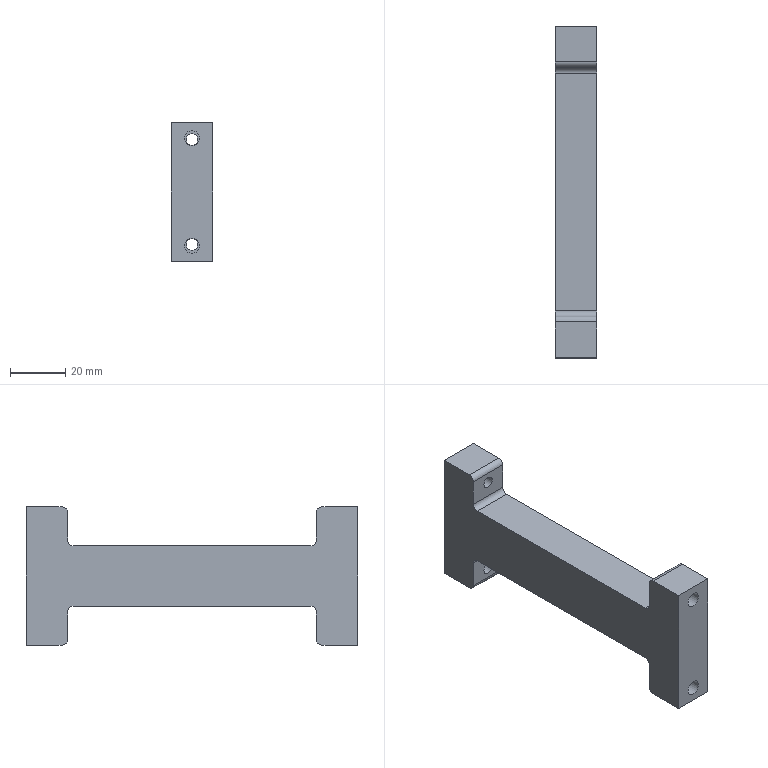Part | STEP file | SynoNew-0304-032 | 1 solid | 26 faces | box 15 x 120 x 50 mm | volume 51097 mm3 | plane 14 | cylinder 12 | commonest cylinder face diameters 4 x8 4.2 x2 5.4 x2
STEP:
#1=CARTESIAN_POINT('',(2.1,60.,6.));
#2=VERTEX_POINT('',#1);
#3=CARTESIAN_POINT('',(-2.1,60.,6.));
#4=VERTEX_POINT('',#3);
#5=CARTESIAN_POINT('',(0.,60.,6.));
#6=DIRECTION('',(0.,-1.,0.));
#7=DIRECTION('',(1.,0.,0.));
#8=AXIS2_PLACEMENT_3D('',#5,#6,#7);
#9=CIRCLE('',#8,2.1);
#10=EDGE_CURVE('',#2,#4,#9,.T.);
#11=ORIENTED_EDGE('',*,*,#10,.F.);
#12=CARTESIAN_POINT('',(0.,60.,6.));
#13=DIRECTION('',(0.,-1.,0.));
#14=DIRECTION('',(1.,0.,0.));
#15=AXIS2_PLACEMENT_3D('',#12,#13,#14);
#16=CIRCLE('',#15,2.1);
#17=EDGE_CURVE('',#4,#2,#16,.T.);
#18=ORIENTED_EDGE('',*,*,#17,.F.);
#19=CARTESIAN_POINT('',(-2.1,45.,6.));
#20=VERTEX_POINT('',#19);
#21=CARTESIAN_POINT('',(-2.1,-70.863,6.));
#22=DIRECTION('',(0.,-1.,0.));
#23=VECTOR('',#22,2.1);
#24=LINE('',#21,#23);
#25=EDGE_CURVE('',#4,#20,#24,.T.);
#26=ORIENTED_EDGE('',*,*,#25,.T.);
#27=CARTESIAN_POINT('',(0.,45.,6.));
#28=DIRECTION('',(0.,1.,0.));
#29=DIRECTION('',(1.,0.,0.));
#30=AXIS2_PLACEMENT_3D('',#27,#28,#29);
#31=CIRCLE('',#30,2.1);
#32=EDGE_CURVE('',#20,#20,#31,.T.);
#33=ORIENTED_EDGE('',*,*,#32,.F.);
#34=ORIENTED_EDGE('',*,*,#25,.F.);
#35=EDGE_LOOP('',(#11,#18,#26,#33,#34));
#36=FACE_OUTER_BOUND('',#35,.T.);
#37=CARTESIAN_POINT('',(0.,-70.863,6.));
#38=DIRECTION('',(0.,1.,0.));
#39=DIRECTION('',(1.,0.,0.));
#40=AXIS2_PLACEMENT_3D('',#37,#38,#39);
#41=CYLINDRICAL_SURFACE('',#40,2.1);
#42=ADVANCED_FACE('',(#36),#41,.F.);
#43=CARTESIAN_POINT('',(2.1,60.,44.));
#44=VERTEX_POINT('',#43);
#45=CARTESIAN_POINT('',(-2.1,60.,44.));
#46=VERTEX_POINT('',#45);
#47=CARTESIAN_POINT('',(0.,60.,44.));
#48=DIRECTION('',(0.,-1.,0.));
#49=DIRECTION('',(1.,0.,0.));
#50=AXIS2_PLACEMENT_3D('',#47,#48,#49);
#51=CIRCLE('',#50,2.1);
#52=EDGE_CURVE('',#44,#46,#51,.T.);
#53=ORIENTED_EDGE('',*,*,#52,.F.);
#54=CARTESIAN_POINT('',(0.,60.,44.));
#55=DIRECTION('',(0.,-1.,0.));
#56=DIRECTION('',(1.,0.,0.));
#57=AXIS2_PLACEMENT_3D('',#54,#55,#56);
#58=CIRCLE('',#57,2.1);
#59=EDGE_CURVE('',#46,#44,#58,.T.);
#60=ORIENTED_EDGE('',*,*,#59,.F.);
#61=CARTESIAN_POINT('',(-2.1,45.,44.));
#62=VERTEX_POINT('',#61);
#63=CARTESIAN_POINT('',(-2.1,-70.863,44.));
#64=DIRECTION('',(0.,-1.,0.));
#65=VECTOR('',#64,2.1);
#66=LINE('',#63,#65);
#67=EDGE_CURVE('',#46,#62,#66,.T.);
#68=ORIENTED_EDGE('',*,*,#67,.T.);
#69=CARTESIAN_POINT('',(0.,45.,44.));
#70=DIRECTION('',(0.,1.,0.));
#71=DIRECTION('',(1.,0.,0.));
#72=AXIS2_PLACEMENT_3D('',#69,#70,#71);
#73=CIRCLE('',#72,2.1);
#74=EDGE_CURVE('',#62,#62,#73,.T.);
#75=ORIENTED_EDGE('',*,*,#74,.F.);
#76=ORIENTED_EDGE('',*,*,#67,.F.);
#77=EDGE_LOOP('',(#53,#60,#68,#75,#76));
#78=FACE_OUTER_BOUND('',#77,.T.);
#79=CARTESIAN_POINT('',(0.,-70.863,44.));
#80=DIRECTION('',(0.,1.,0.));
#81=DIRECTION('',(1.,0.,0.));
#82=AXIS2_PLACEMENT_3D('',#79,#80,#81);
#83=CYLINDRICAL_SURFACE('',#82,2.1);
#84=ADVANCED_FACE('',(#78),#83,.F.);
#85=CARTESIAN_POINT('',(7.5,45.,48.));
#86=VERTEX_POINT('',#85);
#87=CARTESIAN_POINT('',(7.5,47.,50.));
#88=VERTEX_POINT('',#87);
#89=CARTESIAN_POINT('',(7.5,47.,48.));
#90=DIRECTION('',(-1.,0.,0.));
#91=DIRECTION('',(0.,-0.7071,0.7071));
#92=AXIS2_PLACEMENT_3D('',#89,#90,#91);
#93=CIRCLE('',#92,2.);
#94=EDGE_CURVE('',#86,#88,#93,.T.);
#95=ORIENTED_EDGE('',*,*,#94,.T.);
#96=CARTESIAN_POINT('',(-7.5,47.,50.));
#97=VERTEX_POINT('',#96);
#98=CARTESIAN_POINT('',(-3.75,47.,50.));
#99=DIRECTION('',(-1.,0.,0.));
#100=VECTOR('',#99,10.);
#101=LINE('',#98,#100);
#102=EDGE_CURVE('',#88,#97,#101,.T.);
#103=ORIENTED_EDGE('',*,*,#102,.T.);
#104=CARTESIAN_POINT('',(-7.5,45.,48.));
#105=VERTEX_POINT('',#104);
#106=CARTESIAN_POINT('',(-7.5,47.,48.));
#107=DIRECTION('',(1.,0.,0.));
#108=DIRECTION('',(0.,-0.7071,0.7071));
#109=AXIS2_PLACEMENT_3D('',#106,#107,#108);
#110=CIRCLE('',#109,2.);
#111=EDGE_CURVE('',#97,#105,#110,.T.);
#112=ORIENTED_EDGE('',*,*,#111,.T.);
#113=CARTESIAN_POINT('',(-3.75,45.,48.));
#114=DIRECTION('',(1.,0.,0.));
#115=VECTOR('',#114,10.);
#116=LINE('',#113,#115);
#117=EDGE_CURVE('',#105,#86,#116,.T.);
#118=ORIENTED_EDGE('',*,*,#117,.T.);
#119=EDGE_LOOP('',(#95,#103,#112,#118));
#120=FACE_OUTER_BOUND('',#119,.T.);
#121=CARTESIAN_POINT('',(-3.75,47.,48.));
#122=DIRECTION('',(1.,0.,0.));
#123=DIRECTION('',(0.,-0.7071,0.7071));
#124=AXIS2_PLACEMENT_3D('',#121,#122,#123);
#125=CYLINDRICAL_SURFACE('',#124,2.);
#126=ADVANCED_FACE('',(#120),#125,.T.);
#127=ORIENTED_EDGE('',*,*,#102,.F.);
#128=CARTESIAN_POINT('',(7.5,60.,50.));
#129=VERTEX_POINT('',#128);
#130=CARTESIAN_POINT('',(7.5,-60.,50.));
#131=DIRECTION('',(0.,1.,0.));
#132=VECTOR('',#131,10.);
#133=LINE('',#130,#132);
#134=EDGE_CURVE('',#88,#129,#133,.T.);
#135=ORIENTED_EDGE('',*,*,#134,.T.);
#136=CARTESIAN_POINT('',(-7.5,60.,50.));
#137=VERTEX_POINT('',#136);
#138=CARTESIAN_POINT('',(7.5,60.,50.));
#139=DIRECTION('',(-1.,0.,0.));
#140=VECTOR('',#139,10.);
#141=LINE('',#138,#140);
#142=EDGE_CURVE('',#129,#137,#141,.T.);
#143=ORIENTED_EDGE('',*,*,#142,.T.);
#144=CARTESIAN_POINT('',(-7.5,60.,50.));
#145=DIRECTION('',(0.,-1.,0.));
#146=VECTOR('',#145,10.);
#147=LINE('',#144,#146);
#148=EDGE_CURVE('',#137,#97,#147,.T.);
#149=ORIENTED_EDGE('',*,*,#148,.T.);
#150=EDGE_LOOP('',(#127,#135,#143,#149));
#151=FACE_OUTER_BOUND('',#150,.T.);
#152=CARTESIAN_POINT('',(0.,0.,50.));
#153=DIRECTION('',(0.,0.,1.));
#154=DIRECTION('',(1.,0.,0.));
#155=AXIS2_PLACEMENT_3D('',#152,#153,#154);
#156=PLANE('',#155);
#157=ADVANCED_FACE('',(#151),#156,.T.);
#158=ORIENTED_EDGE('',*,*,#94,.F.);
#159=CARTESIAN_POINT('',(7.5,45.,38.));
#160=VERTEX_POINT('',#159);
#161=CARTESIAN_POINT('',(7.5,45.,32.574));
#162=DIRECTION('',(0.,0.,-1.));
#163=VECTOR('',#162,10.);
#164=LINE('',#161,#163);
#165=EDGE_CURVE('',#86,#160,#164,.T.);
#166=ORIENTED_EDGE('',*,*,#165,.T.);
#167=CARTESIAN_POINT('',(7.5,43.,36.));
#168=VERTEX_POINT('',#167);
#169=CARTESIAN_POINT('',(7.5,43.,38.));
#170=DIRECTION('',(1.,0.,0.));
#171=DIRECTION('',(0.,0.7071,-0.7071));
#172=AXIS2_PLACEMENT_3D('',#169,#170,#171);
#173=CIRCLE('',#172,2.);
#174=EDGE_CURVE('',#168,#160,#173,.T.);
#175=ORIENTED_EDGE('',*,*,#174,.F.);
#176=CARTESIAN_POINT('',(7.5,-43.,36.));
#177=VERTEX_POINT('',#176);
#178=CARTESIAN_POINT('',(7.5,-7.5,36.));
#179=DIRECTION('',(0.,-1.,0.));
#180=VECTOR('',#179,10.);
#181=LINE('',#178,#180);
#182=EDGE_CURVE('',#168,#177,#181,.T.);
#183=ORIENTED_EDGE('',*,*,#182,.T.);
#184=CARTESIAN_POINT('',(7.5,-45.,38.));
#185=VERTEX_POINT('',#184);
#186=CARTESIAN_POINT('',(7.5,-43.,38.));
#187=DIRECTION('',(1.,0.,0.));
#188=DIRECTION('',(0.,-0.7071,-0.7071));
#189=AXIS2_PLACEMENT_3D('',#186,#187,#188);
#190=CIRCLE('',#189,2.);
#191=EDGE_CURVE('',#185,#177,#190,.T.);
#192=ORIENTED_EDGE('',*,*,#191,.F.);
#193=CARTESIAN_POINT('',(7.5,-45.,48.));
#194=VERTEX_POINT('',#193);
#195=CARTESIAN_POINT('',(7.5,-45.,18.));
#196=DIRECTION('',(0.,0.,1.));
#197=VECTOR('',#196,10.);
#198=LINE('',#195,#197);
#199=EDGE_CURVE('',#185,#194,#198,.T.);
#200=ORIENTED_EDGE('',*,*,#199,.T.);
#201=CARTESIAN_POINT('',(7.5,-47.,50.));
#202=VERTEX_POINT('',#201);
#203=CARTESIAN_POINT('',(7.5,-47.,48.));
#204=DIRECTION('',(-1.,0.,0.));
#205=DIRECTION('',(0.,0.7071,0.7071));
#206=AXIS2_PLACEMENT_3D('',#203,#204,#205);
#207=CIRCLE('',#206,2.);
#208=EDGE_CURVE('',#202,#194,#207,.T.);
#209=ORIENTED_EDGE('',*,*,#208,.F.);
#210=CARTESIAN_POINT('',(7.5,-60.,50.));
#211=VERTEX_POINT('',#210);
#212=CARTESIAN_POINT('',(7.5,-60.,50.));
#213=DIRECTION('',(0.,1.,0.));
#214=VECTOR('',#213,10.);
#215=LINE('',#212,#214);
#216=EDGE_CURVE('',#211,#202,#215,.T.);
#217=ORIENTED_EDGE('',*,*,#216,.F.);
#218=CARTESIAN_POINT('',(7.5,-60.,0.));
#219=VERTEX_POINT('',#218);
#220=CARTESIAN_POINT('',(7.5,-60.,0.));
#221=DIRECTION('',(0.,0.,1.));
#222=VECTOR('',#221,10.);
#223=LINE('',#220,#222);
#224=EDGE_CURVE('',#219,#211,#223,.T.);
#225=ORIENTED_EDGE('',*,*,#224,.F.);
#226=CARTESIAN_POINT('',(7.5,-47.,0.));
#227=VERTEX_POINT('',#226);
#228=CARTESIAN_POINT('',(7.5,-60.,0.));
#229=DIRECTION('',(0.,1.,0.));
#230=VECTOR('',#229,10.);
#231=LINE('',#228,#230);
#232=EDGE_CURVE('',#219,#227,#231,.T.);
#233=ORIENTED_EDGE('',*,*,#232,.T.);
#234=CARTESIAN_POINT('',(7.5,-45.,2.));
#235=VERTEX_POINT('',#234);
#236=CARTESIAN_POINT('',(7.5,-47.,2.));
#237=DIRECTION('',(-1.,0.,0.));
#238=DIRECTION('',(0.,0.7071,-0.7071));
#239=AXIS2_PLACEMENT_3D('',#236,#237,#238);
#240=CIRCLE('',#239,2.);
#241=EDGE_CURVE('',#235,#227,#240,.T.);
#242=ORIENTED_EDGE('',*,*,#241,.F.);
#243=CARTESIAN_POINT('',(7.5,-45.,12.));
#244=VERTEX_POINT('',#243);
#245=CARTESIAN_POINT('',(7.5,-45.,7.));
#246=DIRECTION('',(0.,0.,1.));
#247=VECTOR('',#246,10.);
#248=LINE('',#245,#247);
#249=EDGE_CURVE('',#235,#244,#248,.T.);
#250=ORIENTED_EDGE('',*,*,#249,.T.);
#251=CARTESIAN_POINT('',(7.5,-43.,14.));
#252=VERTEX_POINT('',#251);
#253=CARTESIAN_POINT('',(7.5,-43.,12.));
#254=DIRECTION('',(1.,0.,0.));
#255=DIRECTION('',(0.,-0.7071,0.7071));
#256=AXIS2_PLACEMENT_3D('',#253,#254,#255);
#257=CIRCLE('',#256,2.);
#258=EDGE_CURVE('',#252,#244,#257,.T.);
#259=ORIENTED_EDGE('',*,*,#258,.F.);
#260=CARTESIAN_POINT('',(7.5,43.,14.));
#261=VERTEX_POINT('',#260);
#262=CARTESIAN_POINT('',(7.5,-7.5,14.));
#263=DIRECTION('',(0.,1.,0.));
#264=VECTOR('',#263,10.);
#265=LINE('',#262,#264);
#266=EDGE_CURVE('',#252,#261,#265,.T.);
#267=ORIENTED_EDGE('',*,*,#266,.T.);
#268=CARTESIAN_POINT('',(7.5,45.,12.));
#269=VERTEX_POINT('',#268);
#270=CARTESIAN_POINT('',(7.5,43.,12.));
#271=DIRECTION('',(1.,0.,0.));
#272=DIRECTION('',(0.,0.7071,0.7071));
#273=AXIS2_PLACEMENT_3D('',#270,#271,#272);
#274=CIRCLE('',#273,2.);
#275=EDGE_CURVE('',#269,#261,#274,.T.);
#276=ORIENTED_EDGE('',*,*,#275,.F.);
#277=CARTESIAN_POINT('',(7.5,45.,2.));
#278=VERTEX_POINT('',#277);
#279=CARTESIAN_POINT('',(7.5,45.,-7.574));
#280=DIRECTION('',(0.,0.,-1.));
#281=VECTOR('',#280,10.);
#282=LINE('',#279,#281);
#283=EDGE_CURVE('',#269,#278,#282,.T.);
#284=ORIENTED_EDGE('',*,*,#283,.T.);
#285=CARTESIAN_POINT('',(7.5,47.,0.));
#286=VERTEX_POINT('',#285);
#287=CARTESIAN_POINT('',(7.5,47.,2.));
#288=DIRECTION('',(-1.,0.,0.));
#289=DIRECTION('',(0.,-0.7071,-0.7071));
#290=AXIS2_PLACEMENT_3D('',#287,#288,#289);
#291=CIRCLE('',#290,2.);
#292=EDGE_CURVE('',#286,#278,#291,.T.);
#293=ORIENTED_EDGE('',*,*,#292,.F.);
#294=CARTESIAN_POINT('',(7.5,60.,0.));
#295=VERTEX_POINT('',#294);
#296=CARTESIAN_POINT('',(7.5,-60.,0.));
#297=DIRECTION('',(0.,1.,0.));
#298=VECTOR('',#297,10.);
#299=LINE('',#296,#298);
#300=EDGE_CURVE('',#286,#295,#299,.T.);
#301=ORIENTED_EDGE('',*,*,#300,.T.);
#302=CARTESIAN_POINT('',(7.5,60.,0.));
#303=DIRECTION('',(0.,0.,1.));
#304=VECTOR('',#303,10.);
#305=LINE('',#302,#304);
#306=EDGE_CURVE('',#295,#129,#305,.T.);
#307=ORIENTED_EDGE('',*,*,#306,.T.);
#308=ORIENTED_EDGE('',*,*,#134,.F.);
#309=EDGE_LOOP('',(#158,#166,#175,#183,#192,#200,#209,#217,#225,#233,#242,#250,#259,#267,#276,#284,#293,#301,#307,#308));
#310=FACE_OUTER_BOUND('',#309,.T.);
#311=CARTESIAN_POINT('',(7.5,-60.,0.));
#312=DIRECTION('',(1.,0.,0.));
#313=DIRECTION('',(0.,1.,0.));
#314=AXIS2_PLACEMENT_3D('',#311,#312,#313);
#315=PLANE('',#314);
#316=ADVANCED_FACE('',(#310),#315,.T.);
#317=CARTESIAN_POINT('',(-7.5,45.,38.));
#318=VERTEX_POINT('',#317);
#319=CARTESIAN_POINT('',(-7.5,43.,36.));
#320=VERTEX_POINT('',#319);
#321=CARTESIAN_POINT('',(-7.5,43.,38.));
#322=DIRECTION('',(-1.,0.,0.));
#323=DIRECTION('',(0.,0.7071,-0.7071));
#324=AXIS2_PLACEMENT_3D('',#321,#322,#323);
#325=CIRCLE('',#324,2.);
#326=EDGE_CURVE('',#318,#320,#325,.T.);
#327=ORIENTED_EDGE('',*,*,#326,.T.);
#328=CARTESIAN_POINT('',(-7.5,43.,36.));
#329=DIRECTION('',(1.,0.,0.));
#330=VECTOR('',#329,10.);
#331=LINE('',#328,#330);
#332=EDGE_CURVE('',#320,#168,#331,.T.);
#333=ORIENTED_EDGE('',*,*,#332,.T.);
#334=ORIENTED_EDGE('',*,*,#174,.T.);
#335=CARTESIAN_POINT('',(-7.5,45.,38.));
#336=DIRECTION('',(-1.,0.,0.));
#337=VECTOR('',#336,10.);
#338=LINE('',#335,#337);
#339=EDGE_CURVE('',#160,#318,#338,.T.);
#340=ORIENTED_EDGE('',*,*,#339,.T.);
#341=EDGE_LOOP('',(#327,#333,#334,#340));
#342=FACE_OUTER_BOUND('',#341,.T.);
#343=CARTESIAN_POINT('',(-7.5,43.,38.));
#344=DIRECTION('',(1.,0.,0.));
#345=DIRECTION('',(0.,0.7071,-0.7071));
#346=AXIS2_PLACEMENT_3D('',#343,#344,#345);
#347=CYLINDRICAL_SURFACE('',#346,2.);
#348=ADVANCED_FACE('',(#342),#347,.F.);
#349=ORIENTED_EDGE('',*,*,#332,.F.);
#350=CARTESIAN_POINT('',(-7.5,-43.,36.));
#351=VERTEX_POINT('',#350);
#352=CARTESIAN_POINT('',(-7.5,52.5,36.));
#353=DIRECTION('',(0.,1.,0.));
#354=VECTOR('',#353,10.);
#355=LINE('',#352,#354);
#356=EDGE_CURVE('',#351,#320,#355,.T.);
#357=ORIENTED_EDGE('',*,*,#356,.F.);
#358=CARTESIAN_POINT('',(-7.5,-43.,36.));
#359=DIRECTION('',(-1.,0.,0.));
#360=VECTOR('',#359,10.);
#361=LINE('',#358,#360);
#362=EDGE_CURVE('',#177,#351,#361,.T.);
#363=ORIENTED_EDGE('',*,*,#362,.F.);
#364=ORIENTED_EDGE('',*,*,#182,.F.);
#365=EDGE_LOOP('',(#349,#357,#363,#364));
#366=FACE_OUTER_BOUND('',#365,.T.);
#367=CARTESIAN_POINT('',(-7.5,45.,36.));
#368=DIRECTION('',(0.,0.,1.));
#369=DIRECTION('',(0.,-1.,0.));
#370=AXIS2_PLACEMENT_3D('',#367,#368,#369);
#371=PLANE('',#370);
#372=ADVANCED_FACE('',(#366),#371,.T.);
#373=CARTESIAN_POINT('',(-7.5,45.,2.));
#374=VERTEX_POINT('',#373);
#375=CARTESIAN_POINT('',(-7.5,47.,0.));
#376=VERTEX_POINT('',#375);
#377=CARTESIAN_POINT('',(-7.5,47.,2.));
#378=DIRECTION('',(1.,0.,0.));
#379=DIRECTION('',(0.,-0.7071,-0.7071));
#380=AXIS2_PLACEMENT_3D('',#377,#378,#379);
#381=CIRCLE('',#380,2.);
#382=EDGE_CURVE('',#374,#376,#381,.T.);
#383=ORIENTED_EDGE('',*,*,#382,.T.);
#384=CARTESIAN_POINT('',(-3.75,47.,0.));
#385=DIRECTION('',(1.,0.,0.));
#386=VECTOR('',#385,10.);
#387=LINE('',#384,#386);
#388=EDGE_CURVE('',#376,#286,#387,.T.);
#389=ORIENTED_EDGE('',*,*,#388,.T.);
#390=ORIENTED_EDGE('',*,*,#292,.T.);
#391=CARTESIAN_POINT('',(-3.75,45.,2.));
#392=DIRECTION('',(-1.,0.,0.));
#393=VECTOR('',#392,10.);
#394=LINE('',#391,#393);
#395=EDGE_CURVE('',#278,#374,#394,.T.);
#396=ORIENTED_EDGE('',*,*,#395,.T.);
#397=EDGE_LOOP('',(#383,#389,#390,#396));
#398=FACE_OUTER_BOUND('',#397,.T.);
#399=CARTESIAN_POINT('',(-3.75,47.,2.));
#400=DIRECTION('',(-1.,0.,0.));
#401=DIRECTION('',(0.,-0.7071,-0.7071));
#402=AXIS2_PLACEMENT_3D('',#399,#400,#401);
#403=CYLINDRICAL_SURFACE('',#402,2.);
#404=ADVANCED_FACE('',(#398),#403,.T.);
#405=ORIENTED_EDGE('',*,*,#111,.F.);
#406=ORIENTED_EDGE('',*,*,#148,.F.);
#407=CARTESIAN_POINT('',(-7.5,60.,0.));
#408=VERTEX_POINT('',#407);
#409=CARTESIAN_POINT('',(-7.5,60.,0.));
#410=DIRECTION('',(0.,0.,1.));
#411=VECTOR('',#410,10.);
#412=LINE('',#409,#411);
#413=EDGE_CURVE('',#408,#137,#412,.T.);
#414=ORIENTED_EDGE('',*,*,#413,.F.);
#415=CARTESIAN_POINT('',(-7.5,60.,0.));
#416=DIRECTION('',(0.,-1.,0.));
#417=VECTOR('',#416,10.);
#418=LINE('',#415,#417);
#419=EDGE_CURVE('',#408,#376,#418,.T.);
#420=ORIENTED_EDGE('',*,*,#419,.T.);
#421=ORIENTED_EDGE('',*,*,#382,.F.);
#422=CARTESIAN_POINT('',(-7.5,45.,12.));
#423=VERTEX_POINT('',#422);
#424=CARTESIAN_POINT('',(-7.5,45.,-7.574));
#425=DIRECTION('',(0.,0.,1.));
#426=VECTOR('',#425,10.);
#427=LINE('',#424,#426);
#428=EDGE_CURVE('',#374,#423,#427,.T.);
#429=ORIENTED_EDGE('',*,*,#428,.T.);
#430=CARTESIAN_POINT('',(-7.5,43.,14.));
#431=VERTEX_POINT('',#430);
#432=CARTESIAN_POINT('',(-7.5,43.,12.));
#433=DIRECTION('',(-1.,0.,0.));
#434=DIRECTION('',(0.,0.7071,0.7071));
#435=AXIS2_PLACEMENT_3D('',#432,#433,#434);
#436=CIRCLE('',#435,2.);
#437=EDGE_CURVE('',#431,#423,#436,.T.);
#438=ORIENTED_EDGE('',*,*,#437,.F.);
#439=CARTESIAN_POINT('',(-7.5,-43.,14.));
#440=VERTEX_POINT('',#439);
#441=CARTESIAN_POINT('',(-7.5,52.5,14.));
#442=DIRECTION('',(0.,-1.,0.));
#443=VECTOR('',#442,10.);
#444=LINE('',#441,#443);
#445=EDGE_CURVE('',#431,#440,#444,.T.);
#446=ORIENTED_EDGE('',*,*,#445,.T.);
#447=CARTESIAN_POINT('',(-7.5,-45.,12.));
#448=VERTEX_POINT('',#447);
#449=CARTESIAN_POINT('',(-7.5,-43.,12.));
#450=DIRECTION('',(-1.,0.,0.));
#451=DIRECTION('',(0.,-0.7071,0.7071));
#452=AXIS2_PLACEMENT_3D('',#449,#450,#451);
#453=CIRCLE('',#452,2.);
#454=EDGE_CURVE('',#448,#440,#453,.T.);
#455=ORIENTED_EDGE('',*,*,#454,.F.);
#456=CARTESIAN_POINT('',(-7.5,-45.,2.));
#457=VERTEX_POINT('',#456);
#458=CARTESIAN_POINT('',(-7.5,-45.,7.));
#459=DIRECTION('',(0.,0.,-1.));
#460=VECTOR('',#459,10.);
#461=LINE('',#458,#460);
#462=EDGE_CURVE('',#448,#457,#461,.T.);
#463=ORIENTED_EDGE('',*,*,#462,.T.);
#464=CARTESIAN_POINT('',(-7.5,-47.,0.));
#465=VERTEX_POINT('',#464);
#466=CARTESIAN_POINT('',(-7.5,-47.,2.));
#467=DIRECTION('',(1.,0.,0.));
#468=DIRECTION('',(0.,0.7071,-0.7071));
#469=AXIS2_PLACEMENT_3D('',#466,#467,#468);
#470=CIRCLE('',#469,2.);
#471=EDGE_CURVE('',#465,#457,#470,.T.);
#472=ORIENTED_EDGE('',*,*,#471,.F.);
#473=CARTESIAN_POINT('',(-7.5,-60.,0.));
#474=VERTEX_POINT('',#473);
#475=CARTESIAN_POINT('',(-7.5,60.,0.));
#476=DIRECTION('',(0.,-1.,0.));
#477=VECTOR('',#476,10.);
#478=LINE('',#475,#477);
#479=EDGE_CURVE('',#465,#474,#478,.T.);
#480=ORIENTED_EDGE('',*,*,#479,.T.);
#481=CARTESIAN_POINT('',(-7.5,-60.,50.));
#482=VERTEX_POINT('',#481);
#483=CARTESIAN_POINT('',(-7.5,-60.,0.));
#484=DIRECTION('',(0.,0.,1.));
#485=VECTOR('',#484,10.);
#486=LINE('',#483,#485);
#487=EDGE_CURVE('',#474,#482,#486,.T.);
#488=ORIENTED_EDGE('',*,*,#487,.T.);
#489=CARTESIAN_POINT('',(-7.5,-47.,50.));
#490=VERTEX_POINT('',#489);
#491=CARTESIAN_POINT('',(-7.5,60.,50.));
#492=DIRECTION('',(0.,-1.,0.));
#493=VECTOR('',#492,10.);
#494=LINE('',#491,#493);
#495=EDGE_CURVE('',#490,#482,#494,.T.);
#496=ORIENTED_EDGE('',*,*,#495,.F.);
#497=CARTESIAN_POINT('',(-7.5,-45.,48.));
#498=VERTEX_POINT('',#497);
#499=CARTESIAN_POINT('',(-7.5,-47.,48.));
#500=DIRECTION('',(1.,0.,0.));
#501=DIRECTION('',(0.,0.7071,0.7071));
#502=AXIS2_PLACEMENT_3D('',#499,#500,#501);
#503=CIRCLE('',#502,2.);
#504=EDGE_CURVE('',#498,#490,#503,.T.);
#505=ORIENTED_EDGE('',*,*,#504,.F.);
#506=CARTESIAN_POINT('',(-7.5,-45.,38.));
#507=VERTEX_POINT('',#506);
#508=CARTESIAN_POINT('',(-7.5,-45.,18.));
#509=DIRECTION('',(0.,0.,-1.));
#510=VECTOR('',#509,10.);
#511=LINE('',#508,#510);
#512=EDGE_CURVE('',#498,#507,#511,.T.);
#513=ORIENTED_EDGE('',*,*,#512,.T.);
#514=CARTESIAN_POINT('',(-7.5,-43.,38.));
#515=DIRECTION('',(-1.,0.,0.));
#516=DIRECTION('',(0.,-0.7071,-0.7071));
#517=AXIS2_PLACEMENT_3D('',#514,#515,#516);
#518=CIRCLE('',#517,2.);
#519=EDGE_CURVE('',#351,#507,#518,.T.);
#520=ORIENTED_EDGE('',*,*,#519,.F.);
#521=ORIENTED_EDGE('',*,*,#356,.T.);
#522=ORIENTED_EDGE('',*,*,#326,.F.);
#523=CARTESIAN_POINT('',(-7.5,45.,32.574));
#524=DIRECTION('',(0.,0.,1.));
#525=VECTOR('',#524,10.);
#526=LINE('',#523,#525);
#527=EDGE_CURVE('',#318,#105,#526,.T.);
#528=ORIENTED_EDGE('',*,*,#527,.T.);
#529=EDGE_LOOP('',(#405,#406,#414,#420,#421,#429,#438,#446,#455,#463,#472,#480,#488,#496,#505,#513,#520,#521,#522,#528));
#530=FACE_OUTER_BOUND('',#529,.T.);
#531=CARTESIAN_POINT('',(-7.5,60.,0.));
#532=DIRECTION('',(-1.,0.,0.));
#533=DIRECTION('',(0.,-1.,0.));
#534=AXIS2_PLACEMENT_3D('',#531,#532,#533);
#535=PLANE('',#534);
#536=ADVANCED_FACE('',(#530),#535,.T.);
#537=ORIENTED_EDGE('',*,*,#395,.F.);
#538=ORIENTED_EDGE('',*,*,#283,.F.);
#539=CARTESIAN_POINT('',(-7.5,45.,12.));
#540=DIRECTION('',(1.,0.,0.));
#541=VECTOR('',#540,10.);
#542=LINE('',#539,#541);
#543=EDGE_CURVE('',#423,#269,#542,.T.);
#544=ORIENTED_EDGE('',*,*,#543,.F.);
#545=ORIENTED_EDGE('',*,*,#428,.F.);
#546=EDGE_LOOP('',(#537,#538,#544,#545));
#547=FACE_OUTER_BOUND('',#546,.T.);
#548=ORIENTED_EDGE('',*,*,#32,.T.);
#549=EDGE_LOOP('',(#548));
#550=FACE_BOUND('',#549,.T.);
#551=CARTESIAN_POINT('',(-7.5,45.,-15.147));
#552=DIRECTION('',(0.,1.,0.));
#553=DIRECTION('',(0.,0.,1.));
#554=AXIS2_PLACEMENT_3D('',#551,#552,#553);
#555=PLANE('',#554);
#556=ADVANCED_FACE('',(#547,#550),#555,.F.);
#557=ORIENTED_EDGE('',*,*,#437,.T.);
#558=ORIENTED_EDGE('',*,*,#543,.T.);
#559=ORIENTED_EDGE('',*,*,#275,.T.);
#560=CARTESIAN_POINT('',(-7.5,43.,14.));
#561=DIRECTION('',(-1.,0.,0.));
#562=VECTOR('',#561,10.);
#563=LINE('',#560,#562);
#564=EDGE_CURVE('',#261,#431,#563,.T.);
#565=ORIENTED_EDGE('',*,*,#564,.T.);
#566=EDGE_LOOP('',(#557,#558,#559,#565));
#567=FACE_OUTER_BOUND('',#566,.T.);
#568=CARTESIAN_POINT('',(-7.5,43.,12.));
#569=DIRECTION('',(1.,0.,0.));
#570=DIRECTION('',(0.,0.7071,0.7071));
#571=AXIS2_PLACEMENT_3D('',#568,#569,#570);
#572=CYLINDRICAL_SURFACE('',#571,2.);
#573=ADVANCED_FACE('',(#567),#572,.F.);
#574=ORIENTED_EDGE('',*,*,#241,.T.);
#575=CARTESIAN_POINT('',(-3.75,-47.,0.));
#576=DIRECTION('',(-1.,0.,0.));
#577=VECTOR('',#576,10.);
#578=LINE('',#575,#577);
#579=EDGE_CURVE('',#227,#465,#578,.T.);
#580=ORIENTED_EDGE('',*,*,#579,.T.);
#581=ORIENTED_EDGE('',*,*,#471,.T.);
#582=CARTESIAN_POINT('',(-3.75,-45.,2.));
#583=DIRECTION('',(1.,0.,0.));
#584=VECTOR('',#583,10.);
#585=LINE('',#582,#584);
#586=EDGE_CURVE('',#457,#235,#585,.T.);
#587=ORIENTED_EDGE('',*,*,#586,.T.);
#588=EDGE_LOOP('',(#574,#580,#581,#587));
#589=FACE_OUTER_BOUND('',#588,.T.);
#590=CARTESIAN_POINT('',(-3.75,-47.,2.));
#591=DIRECTION('',(1.,0.,0.));
#592=DIRECTION('',(0.,0.7071,-0.7071));
#593=AXIS2_PLACEMENT_3D('',#590,#591,#592);
#594=CYLINDRICAL_SURFACE('',#593,2.);
#595=ADVANCED_FACE('',(#589),#594,.T.);
#596=ORIENTED_EDGE('',*,*,#579,.F.);
#597=ORIENTED_EDGE('',*,*,#232,.F.);
#598=CARTESIAN_POINT('',(-7.5,-60.,0.));
#599=DIRECTION('',(1.,0.,0.));
#600=VECTOR('',#599,10.);
#601=LINE('',#598,#600);
#602=EDGE_CURVE('',#474,#219,#601,.T.);
#603=ORIENTED_EDGE('',*,*,#602,.F.);
#604=ORIENTED_EDGE('',*,*,#479,.F.);
#605=EDGE_LOOP('',(#596,#597,#603,#604));
#606=FACE_OUTER_BOUND('',#605,.T.);
#607=CARTESIAN_POINT('',(0.,0.,0.));
#608=DIRECTION('',(0.,0.,1.));
#609=DIRECTION('',(1.,0.,0.));
#610=AXIS2_PLACEMENT_3D('',#607,#608,#609);
#611=PLANE('',#610);
#612=ADVANCED_FACE('',(#606),#611,.F.);
#613=ORIENTED_EDGE('',*,*,#504,.T.);
#614=CARTESIAN_POINT('',(-3.75,-47.,50.));
#615=DIRECTION('',(1.,0.,0.));
#616=VECTOR('',#615,10.);
#617=LINE('',#614,#616);
#618=EDGE_CURVE('',#490,#202,#617,.T.);
#619=ORIENTED_EDGE('',*,*,#618,.T.);
#620=ORIENTED_EDGE('',*,*,#208,.T.);
#621=CARTESIAN_POINT('',(-3.75,-45.,48.));
#622=DIRECTION('',(-1.,0.,0.));
#623=VECTOR('',#622,10.);
#624=LINE('',#621,#623);
#625=EDGE_CURVE('',#194,#498,#624,.T.);
#626=ORIENTED_EDGE('',*,*,#625,.T.);
#627=EDGE_LOOP('',(#613,#619,#620,#626));
#628=FACE_OUTER_BOUND('',#627,.T.);
#629=CARTESIAN_POINT('',(-3.75,-47.,48.));
#630=DIRECTION('',(-1.,0.,0.));
#631=DIRECTION('',(0.,0.7071,0.7071));
#632=AXIS2_PLACEMENT_3D('',#629,#630,#631);
#633=CYLINDRICAL_SURFACE('',#632,2.);
#634=ADVANCED_FACE('',(#628),#633,.T.);
#635=ORIENTED_EDGE('',*,*,#625,.F.);
#636=ORIENTED_EDGE('',*,*,#199,.F.);
#637=CARTESIAN_POINT('',(-7.5,-45.,38.));
#638=DIRECTION('',(1.,0.,0.));
#639=VECTOR('',#638,10.);
#640=LINE('',#637,#639);
#641=EDGE_CURVE('',#507,#185,#640,.T.);
#642=ORIENTED_EDGE('',*,*,#641,.F.);
#643=ORIENTED_EDGE('',*,*,#512,.F.);
#644=EDGE_LOOP('',(#635,#636,#642,#643));
#645=FACE_OUTER_BOUND('',#644,.T.);
#646=CARTESIAN_POINT('',(2.7,-45.,44.5));
#647=VERTEX_POINT('',#646);
#648=CARTESIAN_POINT('',(-2.7,-45.,44.5));
#649=VERTEX_POINT('',#648);
#650=CARTESIAN_POINT('',(0.,-45.,44.5));
#651=DIRECTION('',(0.,-1.,0.));
#652=DIRECTION('',(1.,0.,0.));
#653=AXIS2_PLACEMENT_3D('',#650,#651,#652);
#654=CIRCLE('',#653,2.7);
#655=EDGE_CURVE('',#647,#649,#654,.T.);
#656=ORIENTED_EDGE('',*,*,#655,.T.);
#657=CARTESIAN_POINT('',(0.,-45.,44.5));
#658=DIRECTION('',(0.,-1.,0.));
#659=DIRECTION('',(1.,0.,0.));
#660=AXIS2_PLACEMENT_3D('',#657,#658,#659);
#661=CIRCLE('',#660,2.7);
#662=EDGE_CURVE('',#649,#647,#661,.T.);
#663=ORIENTED_EDGE('',*,*,#662,.T.);
#664=EDGE_LOOP('',(#656,#663));
#665=FACE_BOUND('',#664,.T.);
#666=CARTESIAN_POINT('',(-7.5,-45.,36.));
#667=DIRECTION('',(0.,1.,0.));
#668=DIRECTION('',(0.,0.,1.));
#669=AXIS2_PLACEMENT_3D('',#666,#667,#668);
#670=PLANE('',#669);
#671=ADVANCED_FACE('',(#645,#665),#670,.T.);
#672=ORIENTED_EDGE('',*,*,#519,.T.);
#673=ORIENTED_EDGE('',*,*,#641,.T.);
#674=ORIENTED_EDGE('',*,*,#191,.T.);
#675=ORIENTED_EDGE('',*,*,#362,.T.);
#676=EDGE_LOOP('',(#672,#673,#674,#675));
#677=FACE_OUTER_BOUND('',#676,.T.);
#678=CARTESIAN_POINT('',(-7.5,-43.,38.));
#679=DIRECTION('',(1.,0.,0.));
#680=DIRECTION('',(0.,-0.7071,-0.7071));
#681=AXIS2_PLACEMENT_3D('',#678,#679,#680);
#682=CYLINDRICAL_SURFACE('',#681,2.);
#683=ADVANCED_FACE('',(#677),#682,.F.);
#684=ORIENTED_EDGE('',*,*,#454,.T.);
#685=CARTESIAN_POINT('',(-7.5,-43.,14.));
#686=DIRECTION('',(1.,0.,0.));
#687=VECTOR('',#686,10.);
#688=LINE('',#685,#687);
#689=EDGE_CURVE('',#440,#252,#688,.T.);
#690=ORIENTED_EDGE('',*,*,#689,.T.);
#691=ORIENTED_EDGE('',*,*,#258,.T.);
#692=CARTESIAN_POINT('',(-7.5,-45.,12.));
#693=DIRECTION('',(-1.,0.,0.));
#694=VECTOR('',#693,10.);
#695=LINE('',#692,#694);
#696=EDGE_CURVE('',#244,#448,#695,.T.);
#697=ORIENTED_EDGE('',*,*,#696,.T.);
#698=EDGE_LOOP('',(#684,#690,#691,#697));
#699=FACE_OUTER_BOUND('',#698,.T.);
#700=CARTESIAN_POINT('',(-7.5,-43.,12.));
#701=DIRECTION('',(1.,0.,0.));
#702=DIRECTION('',(0.,-0.7071,0.7071));
#703=AXIS2_PLACEMENT_3D('',#700,#701,#702);
#704=CYLINDRICAL_SURFACE('',#703,2.);
#705=ADVANCED_FACE('',(#699),#704,.F.);
#706=ORIENTED_EDGE('',*,*,#564,.F.);
#707=ORIENTED_EDGE('',*,*,#266,.F.);
#708=ORIENTED_EDGE('',*,*,#689,.F.);
#709=ORIENTED_EDGE('',*,*,#445,.F.);
#710=EDGE_LOOP('',(#706,#707,#708,#709));
#711=FACE_OUTER_BOUND('',#710,.T.);
#712=CARTESIAN_POINT('',(-7.5,45.,14.));
#713=DIRECTION('',(0.,0.,1.));
#714=DIRECTION('',(0.,-1.,0.));
#715=AXIS2_PLACEMENT_3D('',#712,#713,#714);
#716=PLANE('',#715);
#717=ADVANCED_FACE('',(#711),#716,.F.);
#718=CARTESIAN_POINT('',(2.7,-45.,5.5));
#719=VERTEX_POINT('',#718);
#720=CARTESIAN_POINT('',(-2.7,-45.,5.5));
#721=VERTEX_POINT('',#720);
#722=CARTESIAN_POINT('',(0.,-45.,5.5));
#723=DIRECTION('',(0.,-1.,0.));
#724=DIRECTION('',(1.,0.,0.));
#725=AXIS2_PLACEMENT_3D('',#722,#723,#724);
#726=CIRCLE('',#725,2.7);
#727=EDGE_CURVE('',#719,#721,#726,.T.);
#728=ORIENTED_EDGE('',*,*,#727,.F.);
#729=CARTESIAN_POINT('',(0.,-45.,5.5));
#730=DIRECTION('',(0.,-1.,0.));
#731=DIRECTION('',(1.,0.,0.));
#732=AXIS2_PLACEMENT_3D('',#729,#730,#731);
#733=CIRCLE('',#732,2.7);
#734=EDGE_CURVE('',#721,#719,#733,.T.);
#735=ORIENTED_EDGE('',*,*,#734,.F.);
#736=CARTESIAN_POINT('',(-2.7,-60.,5.5));
#737=VERTEX_POINT('',#736);
#738=CARTESIAN_POINT('',(-2.7,-175.863,5.5));
#739=DIRECTION('',(0.,-1.,0.));
#740=VECTOR('',#739,2.7);
#741=LINE('',#738,#740);
#742=EDGE_CURVE('',#721,#737,#741,.T.);
#743=ORIENTED_EDGE('',*,*,#742,.T.);
#744=CARTESIAN_POINT('',(0.,-60.,5.5));
#745=DIRECTION('',(0.,1.,0.));
#746=DIRECTION('',(1.,0.,0.));
#747=AXIS2_PLACEMENT_3D('',#744,#745,#746);
#748=CIRCLE('',#747,2.7);
#749=EDGE_CURVE('',#737,#737,#748,.T.);
#750=ORIENTED_EDGE('',*,*,#749,.F.);
#751=ORIENTED_EDGE('',*,*,#742,.F.);
#752=EDGE_LOOP('',(#728,#735,#743,#750,#751));
#753=FACE_OUTER_BOUND('',#752,.T.);
#754=CARTESIAN_POINT('',(0.,-175.863,5.5));
#755=DIRECTION('',(0.,-1.,0.));
#756=DIRECTION('',(1.,0.,0.));
#757=AXIS2_PLACEMENT_3D('',#754,#755,#756);
#758=CYLINDRICAL_SURFACE('',#757,2.7);
#759=ADVANCED_FACE('',(#753),#758,.F.);
#760=ORIENTED_EDGE('',*,*,#655,.F.);
#761=ORIENTED_EDGE('',*,*,#662,.F.);
#762=CARTESIAN_POINT('',(-2.7,-60.,44.5));
#763=VERTEX_POINT('',#762);
#764=CARTESIAN_POINT('',(-2.7,-175.863,44.5));
#765=DIRECTION('',(0.,-1.,0.));
#766=VECTOR('',#765,2.7);
#767=LINE('',#764,#766);
#768=EDGE_CURVE('',#649,#763,#767,.T.);
#769=ORIENTED_EDGE('',*,*,#768,.T.);
#770=CARTESIAN_POINT('',(0.,-60.,44.5));
#771=DIRECTION('',(0.,1.,0.));
#772=DIRECTION('',(1.,0.,0.));
#773=AXIS2_PLACEMENT_3D('',#770,#771,#772);
#774=CIRCLE('',#773,2.7);
#775=EDGE_CURVE('',#763,#763,#774,.T.);
#776=ORIENTED_EDGE('',*,*,#775,.F.);
#777=ORIENTED_EDGE('',*,*,#768,.F.);
#778=EDGE_LOOP('',(#760,#761,#769,#776,#777));
#779=FACE_OUTER_BOUND('',#778,.T.);
#780=CARTESIAN_POINT('',(0.,-175.863,44.5));
#781=DIRECTION('',(0.,1.,0.));
#782=DIRECTION('',(1.,0.,0.));
#783=AXIS2_PLACEMENT_3D('',#780,#781,#782);
#784=CYLINDRICAL_SURFACE('',#783,2.7);
#785=ADVANCED_FACE('',(#779),#784,.F.);
#786=ORIENTED_EDGE('',*,*,#117,.F.);
#787=ORIENTED_EDGE('',*,*,#527,.F.);
#788=ORIENTED_EDGE('',*,*,#339,.F.);
#789=ORIENTED_EDGE('',*,*,#165,.F.);
#790=EDGE_LOOP('',(#786,#787,#788,#789));
#791=FACE_OUTER_BOUND('',#790,.T.);
#792=ORIENTED_EDGE('',*,*,#74,.T.);
#793=EDGE_LOOP('',(#792));
#794=FACE_BOUND('',#793,.T.);
#795=CARTESIAN_POINT('',(-7.5,45.,65.147));
#796=DIRECTION('',(0.,-1.,0.));
#797=DIRECTION('',(0.,0.,-1.));
#798=AXIS2_PLACEMENT_3D('',#795,#796,#797);
#799=PLANE('',#798);
#800=ADVANCED_FACE('',(#791,#794),#799,.T.);
#801=ORIENTED_EDGE('',*,*,#618,.F.);
#802=ORIENTED_EDGE('',*,*,#495,.T.);
#803=CARTESIAN_POINT('',(-7.5,-60.,50.));
#804=DIRECTION('',(1.,0.,0.));
#805=VECTOR('',#804,10.);
#806=LINE('',#803,#805);
#807=EDGE_CURVE('',#482,#211,#806,.T.);
#808=ORIENTED_EDGE('',*,*,#807,.T.);
#809=ORIENTED_EDGE('',*,*,#216,.T.);
#810=EDGE_LOOP('',(#801,#802,#808,#809));
#811=FACE_OUTER_BOUND('',#810,.T.);
#812=CARTESIAN_POINT('',(0.,0.,50.));
#813=DIRECTION('',(0.,0.,1.));
#814=DIRECTION('',(1.,0.,0.));
#815=AXIS2_PLACEMENT_3D('',#812,#813,#814);
#816=PLANE('',#815);
#817=ADVANCED_FACE('',(#811),#816,.T.);
#818=ORIENTED_EDGE('',*,*,#586,.F.);
#819=ORIENTED_EDGE('',*,*,#462,.F.);
#820=ORIENTED_EDGE('',*,*,#696,.F.);
#821=ORIENTED_EDGE('',*,*,#249,.F.);
#822=EDGE_LOOP('',(#818,#819,#820,#821));
#823=FACE_OUTER_BOUND('',#822,.T.);
#824=ORIENTED_EDGE('',*,*,#727,.T.);
#825=ORIENTED_EDGE('',*,*,#734,.T.);
#826=EDGE_LOOP('',(#824,#825));
#827=FACE_BOUND('',#826,.T.);
#828=CARTESIAN_POINT('',(-7.5,-45.,14.));
#829=DIRECTION('',(0.,-1.,0.));
#830=DIRECTION('',(0.,0.,-1.));
#831=AXIS2_PLACEMENT_3D('',#828,#829,#830);
#832=PLANE('',#831);
#833=ADVANCED_FACE('',(#823,#827),#832,.F.);
#834=ORIENTED_EDGE('',*,*,#388,.F.);
#835=ORIENTED_EDGE('',*,*,#419,.F.);
#836=CARTESIAN_POINT('',(7.5,60.,0.));
#837=DIRECTION('',(-1.,0.,0.));
#838=VECTOR('',#837,10.);
#839=LINE('',#836,#838);
#840=EDGE_CURVE('',#295,#408,#839,.T.);
#841=ORIENTED_EDGE('',*,*,#840,.F.);
#842=ORIENTED_EDGE('',*,*,#300,.F.);
#843=EDGE_LOOP('',(#834,#835,#841,#842));
#844=FACE_OUTER_BOUND('',#843,.T.);
#845=CARTESIAN_POINT('',(0.,0.,0.));
#846=DIRECTION('',(0.,0.,1.));
#847=DIRECTION('',(1.,0.,0.));
#848=AXIS2_PLACEMENT_3D('',#845,#846,#847);
#849=PLANE('',#848);
#850=ADVANCED_FACE('',(#844),#849,.F.);
#851=ORIENTED_EDGE('',*,*,#840,.T.);
#852=ORIENTED_EDGE('',*,*,#413,.T.);
#853=ORIENTED_EDGE('',*,*,#142,.F.);
#854=ORIENTED_EDGE('',*,*,#306,.F.);
#855=EDGE_LOOP('',(#851,#852,#853,#854));
#856=FACE_OUTER_BOUND('',#855,.T.);
#857=ORIENTED_EDGE('',*,*,#10,.T.);
#858=ORIENTED_EDGE('',*,*,#17,.T.);
#859=EDGE_LOOP('',(#857,#858));
#860=FACE_BOUND('',#859,.T.);
#861=ORIENTED_EDGE('',*,*,#52,.T.);
#862=ORIENTED_EDGE('',*,*,#59,.T.);
#863=EDGE_LOOP('',(#861,#862));
#864=FACE_BOUND('',#863,.T.);
#865=CARTESIAN_POINT('',(7.5,60.,0.));
#866=DIRECTION('',(0.,1.,0.));
#867=DIRECTION('',(-1.,0.,0.));
#868=AXIS2_PLACEMENT_3D('',#865,#866,#867);
#869=PLANE('',#868);
#870=ADVANCED_FACE('',(#856,#860,#864),#869,.T.);
#871=ORIENTED_EDGE('',*,*,#602,.T.);
#872=ORIENTED_EDGE('',*,*,#224,.T.);
#873=ORIENTED_EDGE('',*,*,#807,.F.);
#874=ORIENTED_EDGE('',*,*,#487,.F.);
#875=EDGE_LOOP('',(#871,#872,#873,#874));
#876=FACE_OUTER_BOUND('',#875,.T.);
#877=ORIENTED_EDGE('',*,*,#749,.T.);
#878=EDGE_LOOP('',(#877));
#879=FACE_BOUND('',#878,.T.);
#880=ORIENTED_EDGE('',*,*,#775,.T.);
#881=EDGE_LOOP('',(#880));
#882=FACE_BOUND('',#881,.T.);
#883=CARTESIAN_POINT('',(-7.5,-60.,0.));
#884=DIRECTION('',(0.,-1.,0.));
#885=DIRECTION('',(1.,0.,0.));
#886=AXIS2_PLACEMENT_3D('',#883,#884,#885);
#887=PLANE('',#886);
#888=ADVANCED_FACE('',(#876,#879,#882),#887,.T.);
#889=CLOSED_SHELL('',(#42,#84,#126,#157,#316,#348,#372,#404,#536,#556,#573,#595,#612,#634,#671,#683,#705,#717,#759,#785,#800,#817,#833,#850,#870,#888));
#890=MANIFOLD_SOLID_BREP('',#889);
#891=(LENGTH_UNIT()NAMED_UNIT(*)SI_UNIT(.MILLI.,.METRE.));
#892=UNCERTAINTY_MEASURE_WITH_UNIT(LENGTH_MEASURE(0.01),#891,'','');
#893=(NAMED_UNIT(*)PLANE_ANGLE_UNIT()SI_UNIT($,.RADIAN.));
#894=(NAMED_UNIT(*)SI_UNIT($,.STERADIAN.)SOLID_ANGLE_UNIT());
#895=(GEOMETRIC_REPRESENTATION_CONTEXT(3)GLOBAL_UNCERTAINTY_ASSIGNED_CONTEXT((#892))GLOBAL_UNIT_ASSIGNED_CONTEXT((#891,#893,#894))REPRESENTATION_CONTEXT('',''));
#896=ADVANCED_BREP_SHAPE_REPRESENTATION('',(#890),#895);